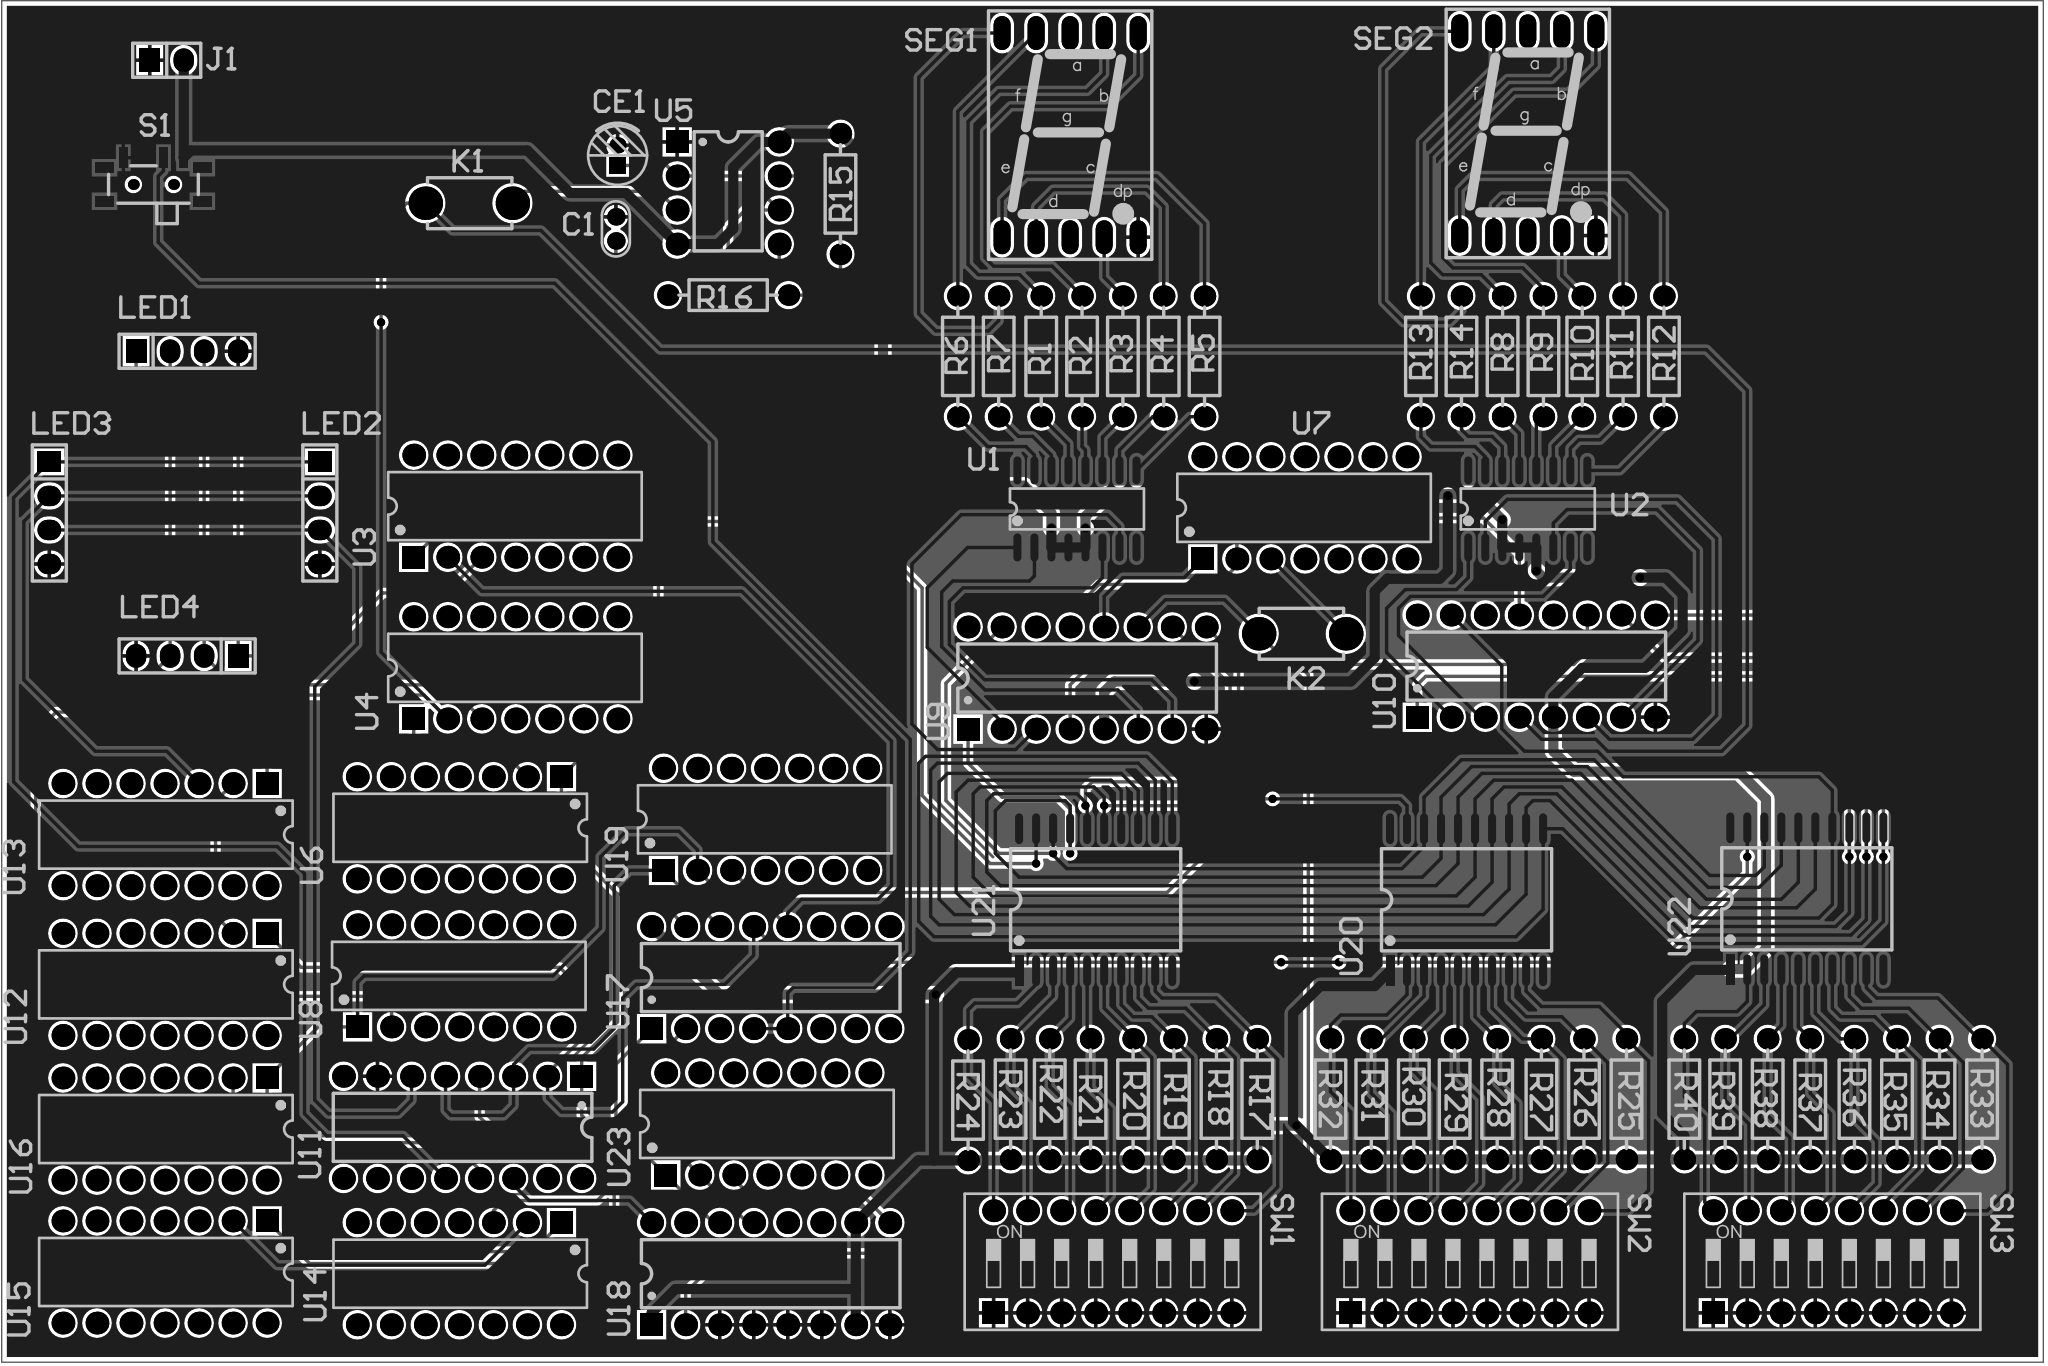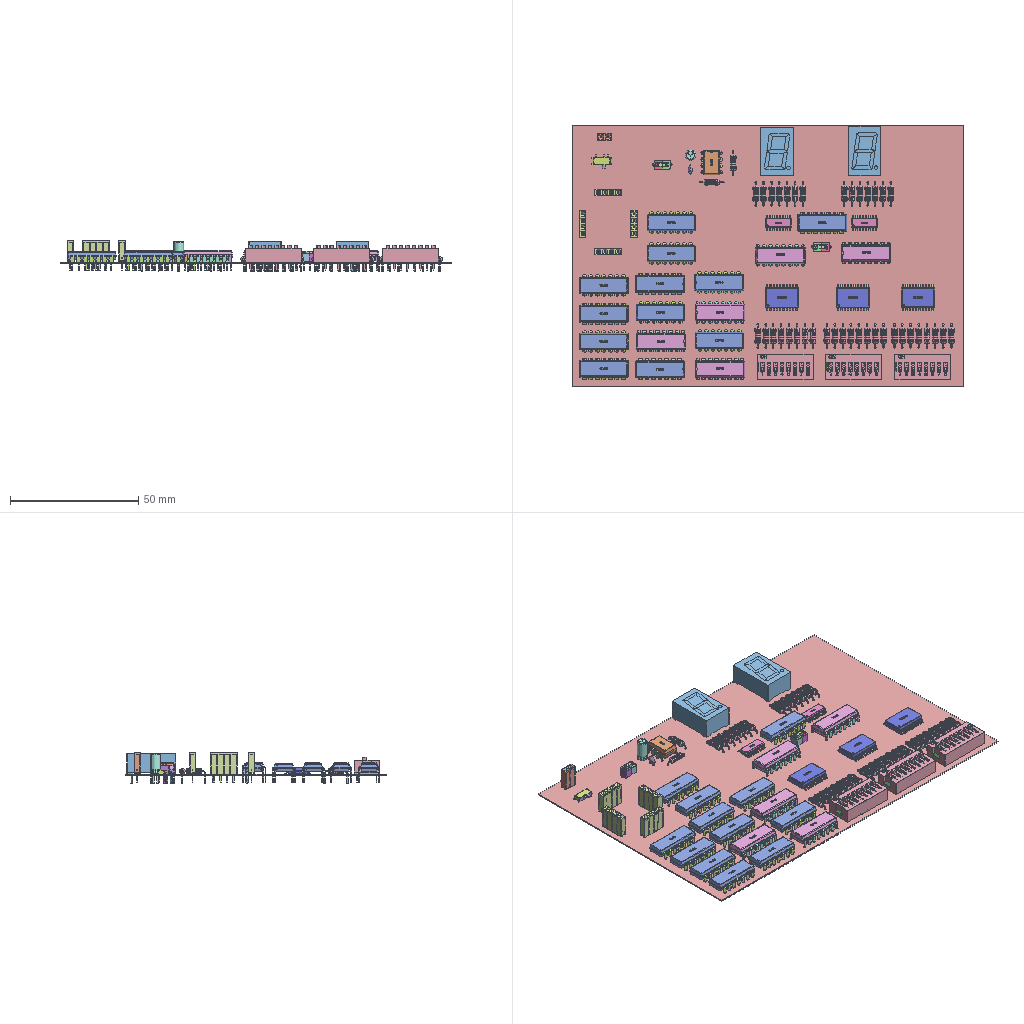Circuit board layout | Altium Designer | box 152.4 x 101.6 x 12.1 mm
Layer stack:
# Altium Designer layer stack of  (unit mm; dielectric type: 0 none, 1 core, 2 prepreg, 3 surface material)
index,name,kind,layer,copper_thickness_mm,dielectric_type,dielectric_thickness_mm,dielectric_material,dielectric_constant
0,Top Paste,other,,,,,,
1,Top Overlay,other,,,,,,
2,Top Solder,dielectric,,,3,0.0102,Solder Resist,3.5
3,Top Layer,copper,Top Layer,0.0356,,,,
4,Dielectric 1,dielectric,,,0,0.32,FR-4,4.8
5,Bottom Layer,copper,Bottom Layer,0.0356,,,,
6,Bottom Solder,dielectric,,,3,0.0102,Solder Resist,3.5
7,Bottom Overlay,other,,,,,,
8,Bottom Paste,other,,,,,,
# drill layer pairs: low layer,high layer
drill_pair,Top Layer,Bottom Layer
Part placement:
Designator,Comment,Layer,Footprint,Center-X(mm),Center-Y(mm),Rotation
U16,74LS04,TopLayer,DIP14,37.592,42.799,270
U15,74LS04,TopLayer,DIP14,37.592,32.131,270
U14,74LS32,TopLayer,DIP14,59.563,32.004,270
U11,DM74ALS11AM,TopLayer,DIP16,59.803,42.926,270
U10,DM74LS192N,TopLayer,DIP16,139.954,77.343,90
K2,KEY,TopLayer,DIP-3X6X4.3,122.48,79.756,180
K1,KEY,TopLayer,DIP-3X6X4.3,60.273,111.887,360
J1,Female HDR1X2,TopLayer,Fe-HDR1X2/2.54-S,37.719,122.555,360
U17,SN74LS138N,TopLayer,DIP16,82.804,54.102,90
U18,SN74LS161D,TopLayer,DIP16,82.804,32.004,90
U21,SN74LS245DW,TopLayer,SOP20,107.061,59.91,90
U1,SN74LS48D,TopLayer,SOP16,105.664,89.073,90
U7,74LS32,TopLayer,DIP14,122.682,89.154,90
U5,NE555P,TopLayer,DIP8,79.629,112.649,0
U6,74LS04,TopLayer,DIP14,59.563,65.278,270
U3,74LS08,TopLayer,DIP14,63.777,89.281,90
U4,74LS08,TopLayer,DIP14,63.777,77.216,90
U8,74LS04,TopLayer,DIP14,59.586,54.229,90
U9,DM74LS192N,TopLayer,DIP16,106.426,76.454,90
U12,74LS04,TopLayer,DIP14,37.592,53.594,270
U13,74LS08,TopLayer,DIP14,37.592,64.77,270
U23,74LS00,TopLayer,DIP14,82.587,43.18,90
U20,SN74LS245DW,TopLayer,SOP20,134.747,59.91,90
U22,SN74LS245DW,TopLayer,SOP20,160.147,59.978,90
U19,74LS08,TopLayer,DIP14,82.423,65.913,90
U2,SN74LS48D,TopLayer,SOP16,139.319,89.073,90
SW1,SW-8P,TopLayer,CSW_DIP-8P,108.331,32.893,360
SW2,SW-8P,TopLayer,CSW_DIP-8P,135.001,32.893,360
SW3,SW-8P,TopLayer,CSW_DIP-8P,162.052,32.893,360
SEG1,0.56IN-1-A,TopLayer,0.56IN-1P,105.156,116.967,0
SEG2,0.56IN-1-A,TopLayer,0.56IN-1P,139.319,117.094,0
S1,SS-12F23,TopLayer,MSK-12C01-07,36.727,113.657,360
R18,200,TopLayer,RS_1/4W,116.078,45.03,270
R19,200,TopLayer,RS_1/4W,112.903,45.03,270
R20,200,TopLayer,RS_1/4W,109.855,45.03,270
R21,200,TopLayer,RS_1/4W,106.68,45.03,270
R22,200,TopLayer,RS_1/4W,103.632,45.03,270
R23,200,TopLayer,RS_1/4W,100.711,45.03,270
R24,200,TopLayer,RS_1/4W,97.536,44.958,270
R17,200,TopLayer,RS_1/4W,119.126,45.03,270
R26,200,TopLayer,RS_1/4W,143.51,45.03,270
R27,200,TopLayer,RS_1/4W,140.335,45.03,270
R28,200,TopLayer,RS_1/4W,137.033,45.03,270
R29,200,TopLayer,RS_1/4W,133.858,45.03,270
R30,200,TopLayer,RS_1/4W,130.81,45.03,270
R31,200,TopLayer,RS_1/4W,127.635,45.03,270
R32,200,TopLayer,RS_1/4W,124.587,45.03,270
R25,200,TopLayer,RS_1/4W,146.685,45.03,270
R34,200,TopLayer,RS_1/4W,170.053,45.03,270
R35,200,TopLayer,RS_1/4W,166.878,45.03,270
R36,200,TopLayer,RS_1/4W,163.703,45.03,270
R37,200,TopLayer,RS_1/4W,160.401,45.03,270
R38,200,TopLayer,RS_1/4W,157.226,45.03,270
R39,200,TopLayer,RS_1/4W,154.051,45.03,270
R40,200,TopLayer,RS_1/4W,151.003,45.03,270
R33,200,TopLayer,RS_1/4W,173.228,45.03,270
R1,200,TopLayer,RS_1/4W,102.997,100.457,90
R2,200,TopLayer,RS_1/4W,106.045,100.457,90
R3,200,TopLayer,RS_1/4W,109.093,100.457,90
R4,200,TopLayer,RS_1/4W,112.141,100.457,90
R5,200,TopLayer,RS_1/4W,115.189,100.457,90
R6,200,TopLayer,RS_1/4W,96.774,100.457,90
R7,200,TopLayer,RS_1/4W,99.822,100.457,90
R8,200,TopLayer,RS_1/4W,137.437,100.457,90
R9,200,TopLayer,RS_1/4W,140.485,100.457,90
R10,200,TopLayer,RS_1/4W,143.383,100.457,90
R11,200,TopLayer,RS_1/4W,146.431,100.457,90
R12,200,TopLayer,RS_1/4W,149.479,100.457,90
R13,200,TopLayer,RS_1/4W,131.341,100.457,90
R14,200,TopLayer,RS_1/4W,134.366,100.457,90
R15,48K,TopLayer,RS_1/4W,88.011,112.577,270
R16,48K,TopLayer,RS_1/4W,79.629,105.029,180
LED1,RGB-3528,TopLayer,Fe-HDR1X4/2.54-S,39.243,100.838,90
LED2,RGB-3528,TopLayer,Fe-HDR1X4/2.54-S,49.149,88.773,0
LED3,RGB-3528,TopLayer,Fe-HDR1X4/2.54-S,28.956,88.773,0
LED4,RGB-3528,TopLayer,Fe-HDR1X4/2.54-S,39.243,78.105,270
CE1,10uF,TopLayer,CAP_1.5*4*8,71.374,115.455,90
C1,10nF,TopLayer,CC_1.8*3.6,71.247,109.971,270
Pad and via stacks:
# Altium Designer via and pad stacks of  (unit mm). Each distinct definition once, with the count of objects using it.
# via: kind,start_layer,end_layer,hole_mm,diameter_mm,mode(0 simple;1 top-mid-bottom;2 full stack),diameter_per_layer,count,example_net
# pad: kind,layer,hole_mm,hole_type(0 round;1 square;2 slot),plating,top_size,top_shape(1 round;2 rect;3 octagon;9 rounded rect),mid_size,bottom_size,mode,footprint,size_per_layer,count,example
pad,Multi-Layer,0.8,0,plated,0.8x0.8,1,0.8x0.8,0.8x0.8,0,MSK-12C01-07,,2,S1.
pad,Multi-Layer,0.8,0,plated,1.7x1.7,1,1.7x1.7,1.7x1.7,0,DIP16,,75,U17.16
pad,Multi-Layer,0.8,0,plated,1.7x1.7,2,1.7x1.7,1.7x1.7,0,DIP16,,5,U17.1
pad,Multi-Layer,1.2,0,plated,2.5x2.5,1,2.5x2.5,2.5x2.5,0,DIP-3X6X4.3,,4,K1.1
pad,Multi-Layer,0.8,0,plated,1.7x1.7,2,1.7x1.7,1.7x1.7,0,DIP14,,12,U15.1
pad,Multi-Layer,0.8,0,plated,1.7x1.7,1,1.7x1.7,1.7x1.7,0,DIP14,,156,U15.2
pad,Multi-Layer,0.8128,0,plated,1.524x1.778,2,1.524x1.778,1.524x1.778,0,Fe-HDR1X2/2.54-S,,1,J1.1
pad,Multi-Layer,0.8128,0,plated,1.524x1.778,1,1.524x1.778,1.524x1.778,0,Fe-HDR1X2/2.54-S,,1,J1.2
pad,Multi-Layer,0.8,0,plated,1.7x1.7,1,1.7x1.7,1.7x1.7,0,DIP8,,7,U5.8
pad,Multi-Layer,0.8,0,plated,1.7x1.7,2,1.7x1.7,1.7x1.7,0,DIP8,,1,U5.1
pad,Multi-Layer,0.85,0,plated,2.54x1.27,1,2.54x1.27,2.54x1.27,0,0.56IN-1P,,20,SEG2.10
pad,Multi-Layer,0.6,0,plated,1.6x1.6,1,1.6x1.6,1.6x1.6,0,RS 1/4W,,80,R14.2
pad,Multi-Layer,0.8128,0,plated,1.524x1.778,1,1.524x1.778,1.524x1.778,0,Fe-HDR1X4/2.54-S,,12,LED1.4
pad,Multi-Layer,0.8128,0,plated,1.524x1.778,2,1.524x1.778,1.524x1.778,0,Fe-HDR1X4/2.54-S,,4,LED1.1
pad,Multi-Layer,0.6,0,plated,1.2x1.2,1,1.2x1.2,1.2x1.2,0,CAP 1.5*4*8,,1,CE1.2
pad,Multi-Layer,0.6,0,plated,1.2x1.2,2,1.2x1.2,1.2x1.2,0,CAP 1.5*4*8,,1,CE1.1
pad,Multi-Layer,0.5,0,plated,1.3x1.3,1,1.3x1.3,1.3x1.3,0,CC 1.8*3.6,,2,C1.2
pad,Multi-Layer,0.9,0,plated,1.7x1.7,1,1.7x1.7,1.7x1.7,0,CSW DIP-8P,,45,SW2.10
pad,Multi-Layer,0.9,0,plated,1.7x1.7,2,1.7x1.7,1.7x1.7,0,CSW DIP-8P,,3,SW2.1
pad,Top Layer,0,0,plated,1.5x0.6,2,1.5x0.6,1.5x0.6,0,MSK-12C01-07,,3,S1.3
pad,Top Layer,0,0,plated,1.4x0.8,2,1.4x0.8,1.4x0.8,0,MSK-12C01-07,,4,S1.0
pad,Top Layer,0,0,plated,0.6x2.1,1,0.6x2.1,0.6x2.1,0,SOP16,,32,U2.1
pad,Top Layer,0,0,plated,2.3x0.6,2,2.3x0.6,2.3x0.6,0,SOP20,,3,U20.1
pad,Top Layer,0,0,plated,2.3x0.6,1,2.3x0.6,2.3x0.6,0,SOP20,,57,U20.2
via,Top Layer,Bottom Layer,0.3048,0.6096,0,,23,NetK1_1
Copper pours:
name,layer,net,type(0 solid;1 hatched;2 none)
D,Bottom Layer,GND,0
D,Top Layer,GND,0
Design rules, without the lines most boards share:
# Altium Designer design rules of  (exported by Altium Designer, unit mm)
# columns: name | kind | enabled | priority | scope1 | scope2 | descriptor | typed fields (field=value)
SilkToSilkClearance | 55 | enabled | 1 | All | All | Silk to Silk (Clearance=0mil) (All),(All) |
SilkToSolderMaskClearance | 54 | enabled | 1 | IsPad | All | Silk To Solder Mask (Clearance=0mil) (IsPad),(All) |
MinimumSolderMaskSliver | 53 | enabled | 1 | All | All | Minimum Solder Mask Sliver (Gap=0mil) (All),(All) |
HoleToHoleClearance | 52 | enabled | 1 | All | All | Hole To Hole Clearance (Gap=10mil) (All),(All) | gap=0.254
DiffPairsRouting | 51 | enabled | 1 | All | All | Differential Pairs Uncoupled Length using the Gap Constraints (Min=10mil) (Max=10mil) (Prefered=10mil)  and Width Constraints (Min=15mil) (Max=15mil) (Prefered=15mil) (All) |
HoleSize | 42 | enabled | 1 | All | All | Hole Size Constraint (Min=1mil) (Max=10000mil) (All) |
SolderMaskExpansion | 13 | enabled | 1 | All | All | Solder Mask Expansion (Expansion =4mil) (All) | expansion=0.1016
PasteMaskExpansion | 14 | enabled | 1 | All | All | Paste Mask Expansion (Expansion =0mil) (All) | expansion=0
RoutingVias | 11 | enabled | 1 | All | All | Routing Via (MinHoleWidth=28mil) (MaxHoleWidth=28mil) (PreferredHoleWidth=28mil) (MinWidth=50mil) (MaxWidth=50mil) (PreferedWidth=50mil) (All) | via_min_hole=0.7112 via_max_hole=0.7112 via_preferred_diameter=1.27 via_preferred_hole=0.7112
Width | 2 | enabled | 1 | All | All | Width Constraint (Min=10mil) (Max=100mil) (Preferred=10mil) (All) |
PolygonConnect | 20 | enabled | 1 | All | All | Polygon Connect Rule(Relief Connect )(Conductor Width=10mil) (Relief Angle=90 Angle) (Entries=4) (Air Gap Width=10mil) (All),(All) | connect_style(0=relief,1=direct,2=none)=0 relief_conductor_width=0.254 relief_entries=4
PlaneConnect | 6 | enabled | 1 | All | All | Power Plane Connect Rule(Relief Connect )(Expansion=20mil) (Conductor Width=10mil) (Air Gap=10mil) (Entries=4) (All) | relief_conductor_width=0.254 relief_entries=4 relief_expansion=0.508
Clearance | 0 | enabled | 1 | All | All | Clearance Constraint (Gap=10mil) (All),(All) | gap=0.254
Classes set for this board:
# Altium Designer classes of  (member kind: 0 net, 1 component, 2 from-to, 3 pad, 4 layer, 5 differential pair, 6 design channel, 7 polygon, 8 structure, 9 xSignal)
# columns: class name | member kind | superclass | members
Sheet1 | 1 | no | LED?; LED?; LED?; R?; R?; R?; R?; R?; R?; R?; R?; R?; R?; R?; R?; R?; R?; R?; R?; R?; R?; R?; R?; R?; R?; R?; R?; R?; R?; R?; R?; R?; R?; R?; R?; R?; R?; R?; R?; R?; R?; R?; SEG?; SW?; SW?; U?; U?; U?; U?; U?; U?; U?; U?; U?; U?; U?; U?; U?; U?; U?; U?; U?; U?; LED1; LED2; LED3; R1; R2; R3; R4; R5; R6; R7; R8; R9; R10; R11; R12; R13; R14; R15; R17; R18; R19; R20; R21; R22; R23; R24; R25; R26; R27; R28; R29; R30; R31; R32; R33; R34; R35; R36; R37; R38; R39; R40; SEG1; SW1; SW2; U1; U8; U9; U18; R6; R13; R23; R34; R40; SEG2; U5; CE1; R2; R9; R16; R19; R30; R36; SW1; U3; U11; U16; LED4; R5; R12; R25; R26; R39; SEG1; U4; U13; LED3; R1; R8; R22; R29; U1; U2; U9; U10; R4; R15; R17; R18; R32; R38; U7; U19; LED2; R11; R21; R28; R35; SW3; U8; U17; R7; R14; R24; R31; R33; S1; U6; U15; C1; LED1; R3; R10; R20; R27; R37; SW2; U12; U14; J1; K1; K2; U20; U21; U22; U23; U4; U22; U7; U13; U3; U17; U20; U12; U6; U23; U21; U5; U19; U18;